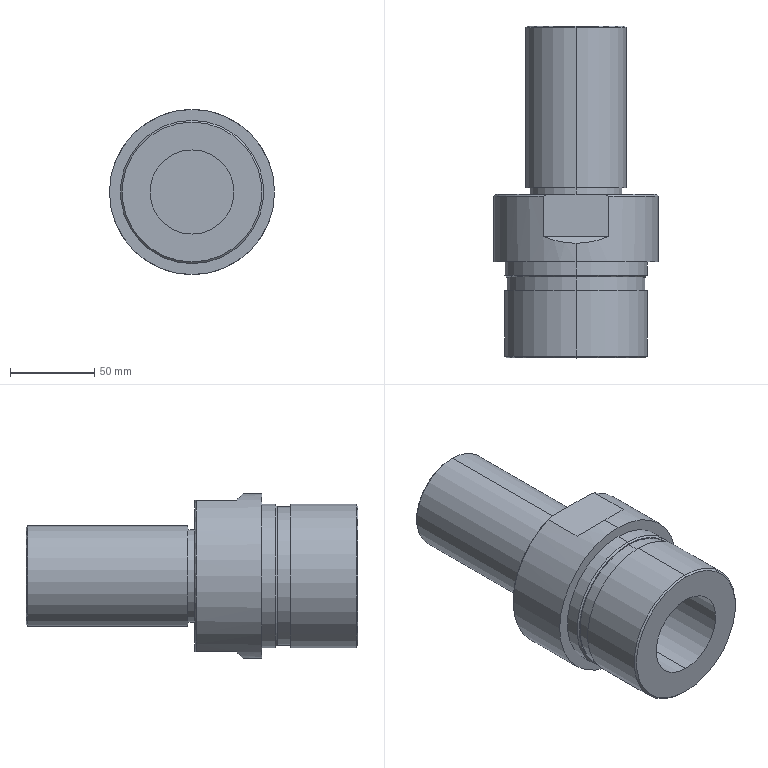Part | SolidWorks | features ICE 11, Chamfer 1, Extrusion 1 | 1 solid | 34 faces | box 98 x 197 x 98 mm | volume 798757 mm3 | cylinder 14 | plane 12 | cone 8 | commonest cylinder face diameters 85 x4 50 x2 55 x2 60 x2 82 x2 98 x2
STEP:
#1=CARTESIAN_POINT('',(0.,-7.,25.));
#2=VERTEX_POINT('',#1);
#3=CARTESIAN_POINT('',(0.,-7.,-25.));
#4=VERTEX_POINT('',#3);
#5=CARTESIAN_POINT('',(0.,-7.,0.));
#6=DIRECTION('',(0.,-1.,0.));
#7=DIRECTION('',(0.,0.,-1.));
#8=AXIS2_PLACEMENT_3D('',#5,#6,#7);
#9=CIRCLE('',#8,25.);
#10=EDGE_CURVE('',#2,#4,#9,.T.);
#11=ORIENTED_EDGE('',*,*,#10,.F.);
#12=CARTESIAN_POINT('',(0.,-57.,25.));
#13=VERTEX_POINT('',#12);
#14=CARTESIAN_POINT('',(0.,-7.,25.));
#15=DIRECTION('',(0.,-1.,0.));
#16=VECTOR('',#15,1000.);
#17=LINE('',#14,#16);
#18=EDGE_CURVE('',#2,#13,#17,.T.);
#19=ORIENTED_EDGE('',*,*,#18,.T.);
#20=CARTESIAN_POINT('',(0.,-57.,-25.));
#21=VERTEX_POINT('',#20);
#22=CARTESIAN_POINT('',(0.,-57.,0.));
#23=DIRECTION('',(0.,-1.,0.));
#24=DIRECTION('',(0.,0.,-1.));
#25=AXIS2_PLACEMENT_3D('',#22,#23,#24);
#26=CIRCLE('',#25,25.);
#27=EDGE_CURVE('',#13,#21,#26,.T.);
#28=ORIENTED_EDGE('',*,*,#27,.T.);
#29=CARTESIAN_POINT('',(0.,-7.,-25.));
#30=DIRECTION('',(0.,-1.,0.));
#31=VECTOR('',#30,1000.);
#32=LINE('',#29,#31);
#33=EDGE_CURVE('',#4,#21,#32,.T.);
#34=ORIENTED_EDGE('',*,*,#33,.F.);
#35=EDGE_LOOP('',(#11,#19,#28,#34));
#36=FACE_OUTER_BOUND('',#35,.T.);
#37=CARTESIAN_POINT('',(0.,-7.,0.));
#38=DIRECTION('',(0.,-1.,0.));
#39=DIRECTION('',(0.,0.,-1.));
#40=AXIS2_PLACEMENT_3D('',#37,#38,#39);
#41=CYLINDRICAL_SURFACE('',#40,25.);
#42=ADVANCED_FACE('',(#36),#41,.F.);
#43=CARTESIAN_POINT('',(0.,139.,-30.));
#44=VERTEX_POINT('',#43);
#45=CARTESIAN_POINT('',(0.,139.,30.));
#46=VERTEX_POINT('',#45);
#47=CARTESIAN_POINT('',(0.,139.,0.));
#48=DIRECTION('',(0.,-1.,0.));
#49=DIRECTION('',(0.,0.,1.));
#50=AXIS2_PLACEMENT_3D('',#47,#48,#49);
#51=CIRCLE('',#50,30.);
#52=EDGE_CURVE('',#44,#46,#51,.T.);
#53=ORIENTED_EDGE('',*,*,#52,.T.);
#54=CARTESIAN_POINT('',(0.,44.,30.));
#55=VERTEX_POINT('',#54);
#56=CARTESIAN_POINT('',(0.,140.,30.));
#57=DIRECTION('',(0.,-1.,0.));
#58=VECTOR('',#57,1000.);
#59=LINE('',#56,#58);
#60=EDGE_CURVE('',#46,#55,#59,.T.);
#61=ORIENTED_EDGE('',*,*,#60,.T.);
#62=CARTESIAN_POINT('',(0.,44.,-30.));
#63=VERTEX_POINT('',#62);
#64=CARTESIAN_POINT('',(0.,44.,0.));
#65=DIRECTION('',(0.,1.,0.));
#66=DIRECTION('',(0.,0.,1.));
#67=AXIS2_PLACEMENT_3D('',#64,#65,#66);
#68=CIRCLE('',#67,30.);
#69=EDGE_CURVE('',#55,#63,#68,.T.);
#70=ORIENTED_EDGE('',*,*,#69,.T.);
#71=CARTESIAN_POINT('',(0.,140.,-30.));
#72=DIRECTION('',(0.,-1.,0.));
#73=VECTOR('',#72,1000.);
#74=LINE('',#71,#73);
#75=EDGE_CURVE('',#44,#63,#74,.T.);
#76=ORIENTED_EDGE('',*,*,#75,.F.);
#77=EDGE_LOOP('',(#53,#61,#70,#76));
#78=FACE_OUTER_BOUND('',#77,.T.);
#79=CARTESIAN_POINT('',(0.,140.,0.));
#80=DIRECTION('',(0.,-1.,0.));
#81=DIRECTION('',(0.,0.,-1.));
#82=AXIS2_PLACEMENT_3D('',#79,#80,#81);
#83=CYLINDRICAL_SURFACE('',#82,30.);
#84=ADVANCED_FACE('',(#78),#83,.T.);
#85=CARTESIAN_POINT('',(0.,140.,29.));
#86=VERTEX_POINT('',#85);
#87=CARTESIAN_POINT('',(0.,140.,-29.));
#88=VERTEX_POINT('',#87);
#89=CARTESIAN_POINT('',(0.,140.,0.));
#90=DIRECTION('',(0.,1.,0.));
#91=DIRECTION('',(0.,0.,1.));
#92=AXIS2_PLACEMENT_3D('',#89,#90,#91);
#93=CIRCLE('',#92,29.);
#94=EDGE_CURVE('',#86,#88,#93,.T.);
#95=ORIENTED_EDGE('',*,*,#94,.F.);
#96=CARTESIAN_POINT('',(0.,140.,29.));
#97=DIRECTION('',(0.,-0.7071,0.7071));
#98=VECTOR('',#97,1000.);
#99=LINE('',#96,#98);
#100=EDGE_CURVE('',#86,#46,#99,.T.);
#101=ORIENTED_EDGE('',*,*,#100,.T.);
#102=ORIENTED_EDGE('',*,*,#52,.F.);
#103=CARTESIAN_POINT('',(0.,140.,-29.));
#104=DIRECTION('',(0.,-0.7071,-0.7071));
#105=VECTOR('',#104,1000.);
#106=LINE('',#103,#105);
#107=EDGE_CURVE('',#88,#44,#106,.T.);
#108=ORIENTED_EDGE('',*,*,#107,.F.);
#109=EDGE_LOOP('',(#95,#101,#102,#108));
#110=FACE_OUTER_BOUND('',#109,.T.);
#111=CARTESIAN_POINT('',(0.,140.,0.));
#112=DIRECTION('',(0.,-1.,0.));
#113=DIRECTION('',(0.,0.,-1.));
#114=AXIS2_PLACEMENT_3D('',#111,#112,#113);
#115=CONICAL_SURFACE('',#114,29.,0.7854);
#116=ADVANCED_FACE('',(#110),#115,.T.);
#117=CARTESIAN_POINT('',(0.,44.,27.5));
#118=VERTEX_POINT('',#117);
#119=CARTESIAN_POINT('',(0.,44.,-27.5));
#120=VERTEX_POINT('',#119);
#121=CARTESIAN_POINT('',(0.,44.,0.));
#122=DIRECTION('',(0.,1.,0.));
#123=DIRECTION('',(0.,0.,1.));
#124=AXIS2_PLACEMENT_3D('',#121,#122,#123);
#125=CIRCLE('',#124,27.5);
#126=EDGE_CURVE('',#118,#120,#125,.T.);
#127=ORIENTED_EDGE('',*,*,#126,.F.);
#128=CARTESIAN_POINT('',(0.,40.,27.5));
#129=VERTEX_POINT('',#128);
#130=CARTESIAN_POINT('',(0.,44.,27.5));
#131=DIRECTION('',(0.,-1.,0.));
#132=VECTOR('',#131,1000.);
#133=LINE('',#130,#132);
#134=EDGE_CURVE('',#118,#129,#133,.T.);
#135=ORIENTED_EDGE('',*,*,#134,.T.);
#136=CARTESIAN_POINT('',(0.,40.,-27.5));
#137=VERTEX_POINT('',#136);
#138=CARTESIAN_POINT('',(0.,40.,0.));
#139=DIRECTION('',(0.,1.,0.));
#140=DIRECTION('',(0.,0.,1.));
#141=AXIS2_PLACEMENT_3D('',#138,#139,#140);
#142=CIRCLE('',#141,27.5);
#143=EDGE_CURVE('',#129,#137,#142,.T.);
#144=ORIENTED_EDGE('',*,*,#143,.T.);
#145=CARTESIAN_POINT('',(0.,44.,-27.5));
#146=DIRECTION('',(0.,-1.,0.));
#147=VECTOR('',#146,1000.);
#148=LINE('',#145,#147);
#149=EDGE_CURVE('',#120,#137,#148,.T.);
#150=ORIENTED_EDGE('',*,*,#149,.F.);
#151=EDGE_LOOP('',(#127,#135,#144,#150));
#152=FACE_OUTER_BOUND('',#151,.T.);
#153=CARTESIAN_POINT('',(0.,44.,0.));
#154=DIRECTION('',(0.,-1.,0.));
#155=DIRECTION('',(0.,0.,-1.));
#156=AXIS2_PLACEMENT_3D('',#153,#154,#155);
#157=CYLINDRICAL_SURFACE('',#156,27.5);
#158=ADVANCED_FACE('',(#152),#157,.T.);
#159=CARTESIAN_POINT('',(0.,-9.,-41.5));
#160=VERTEX_POINT('',#159);
#161=CARTESIAN_POINT('',(0.,-9.,41.5));
#162=VERTEX_POINT('',#161);
#163=CARTESIAN_POINT('',(0.,-9.,0.));
#164=DIRECTION('',(0.,-1.,0.));
#165=DIRECTION('',(0.,0.,-1.));
#166=AXIS2_PLACEMENT_3D('',#163,#164,#165);
#167=CIRCLE('',#166,41.5);
#168=EDGE_CURVE('',#160,#162,#167,.T.);
#169=ORIENTED_EDGE('',*,*,#168,.F.);
#170=CARTESIAN_POINT('',(0.,-8.,-42.5));
#171=VERTEX_POINT('',#170);
#172=CARTESIAN_POINT('',(0.,-9.,-41.5));
#173=DIRECTION('',(0.,0.7071,-0.7071));
#174=VECTOR('',#173,1000.);
#175=LINE('',#172,#174);
#176=EDGE_CURVE('',#160,#171,#175,.T.);
#177=ORIENTED_EDGE('',*,*,#176,.T.);
#178=CARTESIAN_POINT('',(0.,-8.,42.5));
#179=VERTEX_POINT('',#178);
#180=CARTESIAN_POINT('',(0.,-8.,0.));
#181=DIRECTION('',(0.,1.,0.));
#182=DIRECTION('',(0.,0.,-1.));
#183=AXIS2_PLACEMENT_3D('',#180,#181,#182);
#184=CIRCLE('',#183,42.5);
#185=EDGE_CURVE('',#179,#171,#184,.T.);
#186=ORIENTED_EDGE('',*,*,#185,.F.);
#187=CARTESIAN_POINT('',(0.,-9.,41.5));
#188=DIRECTION('',(0.,0.7071,0.7071));
#189=VECTOR('',#188,1000.);
#190=LINE('',#187,#189);
#191=EDGE_CURVE('',#162,#179,#190,.T.);
#192=ORIENTED_EDGE('',*,*,#191,.F.);
#193=EDGE_LOOP('',(#169,#177,#186,#192));
#194=FACE_OUTER_BOUND('',#193,.T.);
#195=CARTESIAN_POINT('',(0.,-9.,0.));
#196=DIRECTION('',(0.,1.,0.));
#197=DIRECTION('',(0.,0.,1.));
#198=AXIS2_PLACEMENT_3D('',#195,#196,#197);
#199=CONICAL_SURFACE('',#198,41.5,0.7854);
#200=ADVANCED_FACE('',(#194),#199,.T.);
#201=CARTESIAN_POINT('',(0.,-57.,-41.5));
#202=VERTEX_POINT('',#201);
#203=CARTESIAN_POINT('',(0.,-57.,41.5));
#204=VERTEX_POINT('',#203);
#205=CARTESIAN_POINT('',(0.,-57.,0.));
#206=DIRECTION('',(0.,-1.,0.));
#207=DIRECTION('',(0.,0.,-1.));
#208=AXIS2_PLACEMENT_3D('',#205,#206,#207);
#209=CIRCLE('',#208,41.5);
#210=EDGE_CURVE('',#202,#204,#209,.T.);
#211=ORIENTED_EDGE('',*,*,#210,.F.);
#212=CARTESIAN_POINT('',(0.,-56.,-42.5));
#213=VERTEX_POINT('',#212);
#214=CARTESIAN_POINT('',(0.,-57.,-41.5));
#215=DIRECTION('',(0.,0.7071,-0.7071));
#216=VECTOR('',#215,1000.);
#217=LINE('',#214,#216);
#218=EDGE_CURVE('',#202,#213,#217,.T.);
#219=ORIENTED_EDGE('',*,*,#218,.T.);
#220=CARTESIAN_POINT('',(0.,-56.,42.5));
#221=VERTEX_POINT('',#220);
#222=CARTESIAN_POINT('',(0.,-56.,0.));
#223=DIRECTION('',(0.,1.,0.));
#224=DIRECTION('',(0.,0.,-1.));
#225=AXIS2_PLACEMENT_3D('',#222,#223,#224);
#226=CIRCLE('',#225,42.5);
#227=EDGE_CURVE('',#221,#213,#226,.T.);
#228=ORIENTED_EDGE('',*,*,#227,.F.);
#229=CARTESIAN_POINT('',(0.,-57.,41.5));
#230=DIRECTION('',(0.,0.7071,0.7071));
#231=VECTOR('',#230,1000.);
#232=LINE('',#229,#231);
#233=EDGE_CURVE('',#204,#221,#232,.T.);
#234=ORIENTED_EDGE('',*,*,#233,.F.);
#235=EDGE_LOOP('',(#211,#219,#228,#234));
#236=FACE_OUTER_BOUND('',#235,.T.);
#237=CARTESIAN_POINT('',(0.,-57.,0.));
#238=DIRECTION('',(0.,1.,0.));
#239=DIRECTION('',(0.,0.,1.));
#240=AXIS2_PLACEMENT_3D('',#237,#238,#239);
#241=CONICAL_SURFACE('',#240,41.5,0.7854);
#242=ADVANCED_FACE('',(#236),#241,.T.);
#243=ORIENTED_EDGE('',*,*,#227,.T.);
#244=CARTESIAN_POINT('',(0.,-17.,-42.5));
#245=VERTEX_POINT('',#244);
#246=CARTESIAN_POINT('',(0.,-57.,-42.5));
#247=DIRECTION('',(0.,1.,0.));
#248=VECTOR('',#247,1000.);
#249=LINE('',#246,#248);
#250=EDGE_CURVE('',#213,#245,#249,.T.);
#251=ORIENTED_EDGE('',*,*,#250,.T.);
#252=CARTESIAN_POINT('',(0.,-17.,42.5));
#253=VERTEX_POINT('',#252);
#254=CARTESIAN_POINT('',(0.,-17.,0.));
#255=DIRECTION('',(0.,-1.,0.));
#256=DIRECTION('',(0.,0.,-1.));
#257=AXIS2_PLACEMENT_3D('',#254,#255,#256);
#258=CIRCLE('',#257,42.5);
#259=EDGE_CURVE('',#245,#253,#258,.T.);
#260=ORIENTED_EDGE('',*,*,#259,.T.);
#261=CARTESIAN_POINT('',(0.,-57.,42.5));
#262=DIRECTION('',(0.,1.,0.));
#263=VECTOR('',#262,1000.);
#264=LINE('',#261,#263);
#265=EDGE_CURVE('',#221,#253,#264,.T.);
#266=ORIENTED_EDGE('',*,*,#265,.F.);
#267=EDGE_LOOP('',(#243,#251,#260,#266));
#268=FACE_OUTER_BOUND('',#267,.T.);
#269=CARTESIAN_POINT('',(0.,-57.,0.));
#270=DIRECTION('',(0.,1.,0.));
#271=DIRECTION('',(0.,0.,1.));
#272=AXIS2_PLACEMENT_3D('',#269,#270,#271);
#273=CYLINDRICAL_SURFACE('',#272,42.5);
#274=ADVANCED_FACE('',(#268),#273,.T.);
#275=CARTESIAN_POINT('',(0.,-17.,-41.));
#276=VERTEX_POINT('',#275);
#277=CARTESIAN_POINT('',(0.,-17.,41.));
#278=VERTEX_POINT('',#277);
#279=CARTESIAN_POINT('',(0.,-17.,0.));
#280=DIRECTION('',(0.,-1.,0.));
#281=DIRECTION('',(0.,0.,-1.));
#282=AXIS2_PLACEMENT_3D('',#279,#280,#281);
#283=CIRCLE('',#282,41.);
#284=EDGE_CURVE('',#276,#278,#283,.T.);
#285=ORIENTED_EDGE('',*,*,#284,.F.);
#286=CARTESIAN_POINT('',(0.,-9.,-41.));
#287=VERTEX_POINT('',#286);
#288=CARTESIAN_POINT('',(0.,-17.,-41.));
#289=DIRECTION('',(0.,1.,0.));
#290=VECTOR('',#289,1000.);
#291=LINE('',#288,#290);
#292=EDGE_CURVE('',#276,#287,#291,.T.);
#293=ORIENTED_EDGE('',*,*,#292,.T.);
#294=CARTESIAN_POINT('',(0.,-9.,41.));
#295=VERTEX_POINT('',#294);
#296=CARTESIAN_POINT('',(0.,-9.,0.));
#297=DIRECTION('',(0.,-1.,0.));
#298=DIRECTION('',(0.,0.,-1.));
#299=AXIS2_PLACEMENT_3D('',#296,#297,#298);
#300=CIRCLE('',#299,41.);
#301=EDGE_CURVE('',#287,#295,#300,.T.);
#302=ORIENTED_EDGE('',*,*,#301,.T.);
#303=CARTESIAN_POINT('',(0.,-17.,41.));
#304=DIRECTION('',(0.,1.,0.));
#305=VECTOR('',#304,1000.);
#306=LINE('',#303,#305);
#307=EDGE_CURVE('',#278,#295,#306,.T.);
#308=ORIENTED_EDGE('',*,*,#307,.F.);
#309=EDGE_LOOP('',(#285,#293,#302,#308));
#310=FACE_OUTER_BOUND('',#309,.T.);
#311=CARTESIAN_POINT('',(0.,-17.,0.));
#312=DIRECTION('',(0.,1.,0.));
#313=DIRECTION('',(0.,0.,1.));
#314=AXIS2_PLACEMENT_3D('',#311,#312,#313);
#315=CYLINDRICAL_SURFACE('',#314,41.);
#316=ADVANCED_FACE('',(#310),#315,.T.);
#317=ORIENTED_EDGE('',*,*,#185,.T.);
#318=CARTESIAN_POINT('',(0.,0.,-42.5));
#319=VERTEX_POINT('',#318);
#320=CARTESIAN_POINT('',(0.,-9.,-42.5));
#321=DIRECTION('',(0.,1.,0.));
#322=VECTOR('',#321,1000.);
#323=LINE('',#320,#322);
#324=EDGE_CURVE('',#171,#319,#323,.T.);
#325=ORIENTED_EDGE('',*,*,#324,.T.);
#326=CARTESIAN_POINT('',(0.,0.,42.5));
#327=VERTEX_POINT('',#326);
#328=CARTESIAN_POINT('',(0.,0.,0.));
#329=DIRECTION('',(0.,-1.,0.));
#330=DIRECTION('',(0.,0.,1.));
#331=AXIS2_PLACEMENT_3D('',#328,#329,#330);
#332=CIRCLE('',#331,42.5);
#333=EDGE_CURVE('',#319,#327,#332,.T.);
#334=ORIENTED_EDGE('',*,*,#333,.T.);
#335=CARTESIAN_POINT('',(0.,-9.,42.5));
#336=DIRECTION('',(0.,1.,0.));
#337=VECTOR('',#336,1000.);
#338=LINE('',#335,#337);
#339=EDGE_CURVE('',#179,#327,#338,.T.);
#340=ORIENTED_EDGE('',*,*,#339,.F.);
#341=EDGE_LOOP('',(#317,#325,#334,#340));
#342=FACE_OUTER_BOUND('',#341,.T.);
#343=CARTESIAN_POINT('',(0.,-9.,0.));
#344=DIRECTION('',(0.,1.,0.));
#345=DIRECTION('',(0.,0.,1.));
#346=AXIS2_PLACEMENT_3D('',#343,#344,#345);
#347=CYLINDRICAL_SURFACE('',#346,42.5);
#348=ADVANCED_FACE('',(#342),#347,.T.);
#349=CARTESIAN_POINT('',(19.391,15.,45.));
#350=VERTEX_POINT('',#349);
#351=CARTESIAN_POINT('',(0.,11.,49.));
#352=VERTEX_POINT('',#351);
#353=CARTESIAN_POINT('',(19.391,15.,45.));
#354=CARTESIAN_POINT('',(13.245,12.352,47.648));
#355=CARTESIAN_POINT('',(6.692,11.,49.));
#356=CARTESIAN_POINT('',(0.,11.,49.));
#357=(BOUNDED_CURVE()B_SPLINE_CURVE(3,(#353,#354,#355,#356),.UNSPECIFIED.,.F.,.F.)B_SPLINE_CURVE_WITH_KNOTS((4,4),(5.876,6.283),.UNSPECIFIED.)CURVE()GEOMETRIC_REPRESENTATION_ITEM()RATIONAL_B_SPLINE_CURVE((1.,0.9863,0.9863,1.))REPRESENTATION_ITEM(''));
#358=EDGE_CURVE('',#350,#352,#357,.T.);
#359=ORIENTED_EDGE('',*,*,#358,.T.);
#360=CARTESIAN_POINT('',(0.,0.,49.));
#361=VERTEX_POINT('',#360);
#362=CARTESIAN_POINT('',(0.,40.,49.));
#363=DIRECTION('',(0.,-1.,0.));
#364=VECTOR('',#363,1000.);
#365=LINE('',#362,#364);
#366=EDGE_CURVE('',#352,#361,#365,.T.);
#367=ORIENTED_EDGE('',*,*,#366,.T.);
#368=CARTESIAN_POINT('',(0.,0.,-49.));
#369=VERTEX_POINT('',#368);
#370=CARTESIAN_POINT('',(0.,0.,0.));
#371=DIRECTION('',(0.,1.,0.));
#372=DIRECTION('',(0.,0.,1.));
#373=AXIS2_PLACEMENT_3D('',#370,#371,#372);
#374=CIRCLE('',#373,49.);
#375=EDGE_CURVE('',#361,#369,#374,.T.);
#376=ORIENTED_EDGE('',*,*,#375,.T.);
#377=CARTESIAN_POINT('',(0.,11.,-49.));
#378=VERTEX_POINT('',#377);
#379=CARTESIAN_POINT('',(0.,40.,-49.));
#380=DIRECTION('',(0.,-1.,0.));
#381=VECTOR('',#380,1000.);
#382=LINE('',#379,#381);
#383=EDGE_CURVE('',#378,#369,#382,.T.);
#384=ORIENTED_EDGE('',*,*,#383,.F.);
#385=CARTESIAN_POINT('',(19.391,15.,-45.));
#386=VERTEX_POINT('',#385);
#387=CARTESIAN_POINT('',(0.,11.,-49.));
#388=CARTESIAN_POINT('',(6.692,11.,-49.));
#389=CARTESIAN_POINT('',(13.245,12.352,-47.648));
#390=CARTESIAN_POINT('',(19.391,15.,-45.));
#391=(BOUNDED_CURVE()B_SPLINE_CURVE(3,(#387,#388,#389,#390),.UNSPECIFIED.,.F.,.F.)B_SPLINE_CURVE_WITH_KNOTS((4,4),(0.,0.4069),.UNSPECIFIED.)CURVE()GEOMETRIC_REPRESENTATION_ITEM()RATIONAL_B_SPLINE_CURVE((1.,0.9863,0.9863,1.))REPRESENTATION_ITEM(''));
#392=EDGE_CURVE('',#378,#386,#391,.T.);
#393=ORIENTED_EDGE('',*,*,#392,.T.);
#394=CARTESIAN_POINT('',(19.391,39.,-45.));
#395=VERTEX_POINT('',#394);
#396=CARTESIAN_POINT('',(19.391,40.,-45.));
#397=DIRECTION('',(0.,1.,0.));
#398=VECTOR('',#397,1000.);
#399=LINE('',#396,#398);
#400=EDGE_CURVE('',#386,#395,#399,.T.);
#401=ORIENTED_EDGE('',*,*,#400,.T.);
#402=CARTESIAN_POINT('',(19.391,39.,45.));
#403=VERTEX_POINT('',#402);
#404=CARTESIAN_POINT('',(0.,39.,0.));
#405=DIRECTION('',(0.,-1.,0.));
#406=DIRECTION('',(0.,0.,1.));
#407=AXIS2_PLACEMENT_3D('',#404,#405,#406);
#408=CIRCLE('',#407,49.);
#409=EDGE_CURVE('',#395,#403,#408,.T.);
#410=ORIENTED_EDGE('',*,*,#409,.T.);
#411=CARTESIAN_POINT('',(19.391,40.,45.));
#412=DIRECTION('',(0.,-1.,0.));
#413=VECTOR('',#412,1000.);
#414=LINE('',#411,#413);
#415=EDGE_CURVE('',#403,#350,#414,.T.);
#416=ORIENTED_EDGE('',*,*,#415,.T.);
#417=EDGE_LOOP('',(#359,#367,#376,#384,#393,#401,#410,#416));
#418=FACE_OUTER_BOUND('',#417,.T.);
#419=CARTESIAN_POINT('',(0.,40.,0.));
#420=DIRECTION('',(0.,-1.,0.));
#421=DIRECTION('',(0.,0.,-1.));
#422=AXIS2_PLACEMENT_3D('',#419,#420,#421);
#423=CYLINDRICAL_SURFACE('',#422,49.);
#424=ADVANCED_FACE('',(#418),#423,.T.);
#425=ORIENTED_EDGE('',*,*,#366,.F.);
#426=CARTESIAN_POINT('',(-19.391,15.,45.));
#427=VERTEX_POINT('',#426);
#428=CARTESIAN_POINT('',(0.,11.,49.));
#429=CARTESIAN_POINT('',(-6.692,11.,49.));
#430=CARTESIAN_POINT('',(-13.245,12.352,47.648));
#431=CARTESIAN_POINT('',(-19.391,15.,45.));
#432=(BOUNDED_CURVE()B_SPLINE_CURVE(3,(#428,#429,#430,#431),.UNSPECIFIED.,.F.,.F.)B_SPLINE_CURVE_WITH_KNOTS((4,4),(0.,0.4069),.UNSPECIFIED.)CURVE()GEOMETRIC_REPRESENTATION_ITEM()RATIONAL_B_SPLINE_CURVE((1.,0.9863,0.9863,1.))REPRESENTATION_ITEM(''));
#433=EDGE_CURVE('',#352,#427,#432,.T.);
#434=ORIENTED_EDGE('',*,*,#433,.T.);
#435=CARTESIAN_POINT('',(-19.391,39.,45.));
#436=VERTEX_POINT('',#435);
#437=CARTESIAN_POINT('',(-19.391,40.,45.));
#438=DIRECTION('',(0.,1.,0.));
#439=VECTOR('',#438,1000.);
#440=LINE('',#437,#439);
#441=EDGE_CURVE('',#427,#436,#440,.T.);
#442=ORIENTED_EDGE('',*,*,#441,.T.);
#443=CARTESIAN_POINT('',(-19.391,39.,-45.));
#444=VERTEX_POINT('',#443);
#445=CARTESIAN_POINT('',(0.,39.,0.));
#446=DIRECTION('',(0.,-1.,0.));
#447=DIRECTION('',(0.,0.,1.));
#448=AXIS2_PLACEMENT_3D('',#445,#446,#447);
#449=CIRCLE('',#448,49.);
#450=EDGE_CURVE('',#436,#444,#449,.T.);
#451=ORIENTED_EDGE('',*,*,#450,.T.);
#452=CARTESIAN_POINT('',(-19.391,15.,-45.));
#453=VERTEX_POINT('',#452);
#454=CARTESIAN_POINT('',(-19.391,40.,-45.));
#455=DIRECTION('',(0.,-1.,0.));
#456=VECTOR('',#455,1000.);
#457=LINE('',#454,#456);
#458=EDGE_CURVE('',#444,#453,#457,.T.);
#459=ORIENTED_EDGE('',*,*,#458,.T.);
#460=CARTESIAN_POINT('',(-19.391,15.,-45.));
#461=CARTESIAN_POINT('',(-13.245,12.352,-47.648));
#462=CARTESIAN_POINT('',(-6.692,11.,-49.));
#463=CARTESIAN_POINT('',(0.,11.,-49.));
#464=(BOUNDED_CURVE()B_SPLINE_CURVE(3,(#460,#461,#462,#463),.UNSPECIFIED.,.F.,.F.)B_SPLINE_CURVE_WITH_KNOTS((4,4),(5.876,6.283),.UNSPECIFIED.)CURVE()GEOMETRIC_REPRESENTATION_ITEM()RATIONAL_B_SPLINE_CURVE((1.,0.9863,0.9863,1.))REPRESENTATION_ITEM(''));
#465=EDGE_CURVE('',#453,#378,#464,.T.);
#466=ORIENTED_EDGE('',*,*,#465,.T.);
#467=ORIENTED_EDGE('',*,*,#383,.T.);
#468=CARTESIAN_POINT('',(0.,0.,0.));
#469=DIRECTION('',(0.,1.,0.));
#470=DIRECTION('',(0.,0.,1.));
#471=AXIS2_PLACEMENT_3D('',#468,#469,#470);
#472=CIRCLE('',#471,49.);
#473=EDGE_CURVE('',#369,#361,#472,.T.);
#474=ORIENTED_EDGE('',*,*,#473,.T.);
#475=EDGE_LOOP('',(#425,#434,#442,#451,#459,#466,#467,#474));
#476=FACE_OUTER_BOUND('',#475,.T.);
#477=CARTESIAN_POINT('',(0.,40.,0.));
#478=DIRECTION('',(0.,-1.,0.));
#479=DIRECTION('',(0.,0.,-1.));
#480=AXIS2_PLACEMENT_3D('',#477,#478,#479);
#481=CYLINDRICAL_SURFACE('',#480,49.);
#482=ADVANCED_FACE('',(#476),#481,.T.);
#483=CARTESIAN_POINT('',(16.703,40.,45.));
#484=VERTEX_POINT('',#483);
#485=CARTESIAN_POINT('',(19.391,39.,45.));
#486=CARTESIAN_POINT('',(18.502,39.352,45.));
#487=CARTESIAN_POINT('',(17.607,39.686,45.));
#488=CARTESIAN_POINT('',(16.703,40.,45.));
#489=B_SPLINE_CURVE_WITH_KNOTS('',3,(#485,#486,#487,#488),.UNSPECIFIED.,.F.,.F.,(4,4),(0.09858,0.1015),.UNSPECIFIED.);
#490=EDGE_CURVE('',#403,#484,#489,.T.);
#491=ORIENTED_EDGE('',*,*,#490,.F.);
#492=ORIENTED_EDGE('',*,*,#409,.F.);
#493=CARTESIAN_POINT('',(16.703,40.,-45.));
#494=VERTEX_POINT('',#493);
#495=CARTESIAN_POINT('',(16.703,40.,-45.));
#496=CARTESIAN_POINT('',(17.604,39.687,-45.));
#497=CARTESIAN_POINT('',(18.5,39.353,-45.));
#498=CARTESIAN_POINT('',(19.391,39.,-45.));
#499=B_SPLINE_CURVE_WITH_KNOTS('',3,(#495,#496,#497,#498),.UNSPECIFIED.,.F.,.F.,(4,4),(0.1355,0.1384),.UNSPECIFIED.);
#500=EDGE_CURVE('',#494,#395,#499,.T.);
#501=ORIENTED_EDGE('',*,*,#500,.F.);
#502=CARTESIAN_POINT('',(0.,40.,0.));
#503=DIRECTION('',(0.,1.,0.));
#504=DIRECTION('',(0.,0.,1.));
#505=AXIS2_PLACEMENT_3D('',#502,#503,#504);
#506=CIRCLE('',#505,48.);
#507=EDGE_CURVE('',#484,#494,#506,.T.);
#508=ORIENTED_EDGE('',*,*,#507,.F.);
#509=EDGE_LOOP('',(#491,#492,#501,#508));
#510=FACE_OUTER_BOUND('',#509,.T.);
#511=CARTESIAN_POINT('',(0.,40.,0.));
#512=DIRECTION('',(0.,-1.,0.));
#513=DIRECTION('',(0.,0.,-1.));
#514=AXIS2_PLACEMENT_3D('',#511,#512,#513);
#515=CONICAL_SURFACE('',#514,48.,0.7854);
#516=ADVANCED_FACE('',(#510),#515,.T.);
#517=CARTESIAN_POINT('',(0.,-9.,0.));
#518=DIRECTION('',(0.,-1.,0.));
#519=DIRECTION('',(0.,0.,-1.));
#520=AXIS2_PLACEMENT_3D('',#517,#518,#519);
#521=CIRCLE('',#520,41.5);
#522=EDGE_CURVE('',#162,#160,#521,.T.);
#523=ORIENTED_EDGE('',*,*,#522,.T.);
#524=ORIENTED_EDGE('',*,*,#168,.T.);
#525=EDGE_LOOP('',(#523,#524));
#526=FACE_OUTER_BOUND('',#525,.T.);
#527=CARTESIAN_POINT('',(0.,-9.,0.));
#528=DIRECTION('',(0.,-1.,0.));
#529=DIRECTION('',(0.,0.,-1.));
#530=AXIS2_PLACEMENT_3D('',#527,#528,#529);
#531=CIRCLE('',#530,41.);
#532=EDGE_CURVE('',#295,#287,#531,.T.);
#533=ORIENTED_EDGE('',*,*,#532,.F.);
#534=ORIENTED_EDGE('',*,*,#301,.F.);
#535=EDGE_LOOP('',(#533,#534));
#536=FACE_BOUND('',#535,.T.);
#537=CARTESIAN_POINT('',(0.,-9.,0.));
#538=DIRECTION('',(0.,-1.,0.));
#539=DIRECTION('',(0.,0.,-1.));
#540=AXIS2_PLACEMENT_3D('',#537,#538,#539);
#541=PLANE('',#540);
#542=ADVANCED_FACE('',(#526,#536),#541,.T.);
#543=ORIENTED_EDGE('',*,*,#473,.F.);
#544=ORIENTED_EDGE('',*,*,#375,.F.);
#545=EDGE_LOOP('',(#543,#544));
#546=FACE_OUTER_BOUND('',#545,.T.);
#547=CARTESIAN_POINT('',(0.,0.,0.));
#548=DIRECTION('',(0.,-1.,0.));
#549=DIRECTION('',(0.,0.,1.));
#550=AXIS2_PLACEMENT_3D('',#547,#548,#549);
#551=CIRCLE('',#550,42.5);
#552=EDGE_CURVE('',#327,#319,#551,.T.);
#553=ORIENTED_EDGE('',*,*,#552,.F.);
#554=ORIENTED_EDGE('',*,*,#333,.F.);
#555=EDGE_LOOP('',(#553,#554));
#556=FACE_BOUND('',#555,.T.);
#557=CARTESIAN_POINT('',(0.,0.,0.));
#558=DIRECTION('',(0.,1.,0.));
#559=DIRECTION('',(0.,0.,1.));
#560=AXIS2_PLACEMENT_3D('',#557,#558,#559);
#561=PLANE('',#560);
#562=ADVANCED_FACE('',(#546,#556),#561,.F.);
#563=CARTESIAN_POINT('',(-16.703,40.,45.));
#564=VERTEX_POINT('',#563);
#565=CARTESIAN_POINT('',(-77.,40.,45.));
#566=DIRECTION('',(-1.,0.,0.));
#567=VECTOR('',#566,1000.);
#568=LINE('',#565,#567);
#569=EDGE_CURVE('',#484,#564,#568,.T.);
#570=ORIENTED_EDGE('',*,*,#569,.F.);
#571=ORIENTED_EDGE('',*,*,#507,.T.);
#572=CARTESIAN_POINT('',(-16.703,40.,-45.));
#573=VERTEX_POINT('',#572);
#574=CARTESIAN_POINT('',(-77.,40.,-45.));
#575=DIRECTION('',(1.,0.,0.));
#576=VECTOR('',#575,1000.);
#577=LINE('',#574,#576);
#578=EDGE_CURVE('',#573,#494,#577,.T.);
#579=ORIENTED_EDGE('',*,*,#578,.F.);
#580=CARTESIAN_POINT('',(0.,40.,0.));
#581=DIRECTION('',(0.,1.,0.));
#582=DIRECTION('',(0.,0.,1.));
#583=AXIS2_PLACEMENT_3D('',#580,#581,#582);
#584=CIRCLE('',#583,48.);
#585=EDGE_CURVE('',#573,#564,#584,.T.);
#586=ORIENTED_EDGE('',*,*,#585,.T.);
#587=EDGE_LOOP('',(#570,#571,#579,#586));
#588=FACE_OUTER_BOUND('',#587,.T.);
#589=CARTESIAN_POINT('',(0.,40.,0.));
#590=DIRECTION('',(0.,1.,0.));
#591=DIRECTION('',(0.,0.,1.));
#592=AXIS2_PLACEMENT_3D('',#589,#590,#591);
#593=CIRCLE('',#592,27.5);
#594=EDGE_CURVE('',#137,#129,#593,.T.);
#595=ORIENTED_EDGE('',*,*,#594,.F.);
#596=ORIENTED_EDGE('',*,*,#143,.F.);
#597=EDGE_LOOP('',(#595,#596));
#598=FACE_BOUND('',#597,.T.);
#599=CARTESIAN_POINT('',(0.,40.,0.));
#600=DIRECTION('',(0.,1.,0.));
#601=DIRECTION('',(0.,0.,1.));
#602=AXIS2_PLACEMENT_3D('',#599,#600,#601);
#603=PLANE('',#602);
#604=ADVANCED_FACE('',(#588,#598),#603,.T.);
#605=ORIENTED_EDGE('',*,*,#324,.F.);
#606=CARTESIAN_POINT('',(0.,-8.,0.));
#607=DIRECTION('',(0.,1.,0.));
#608=DIRECTION('',(0.,0.,-1.));
#609=AXIS2_PLACEMENT_3D('',#606,#607,#608);
#610=CIRCLE('',#609,42.5);
#611=EDGE_CURVE('',#171,#179,#610,.T.);
#612=ORIENTED_EDGE('',*,*,#611,.T.);
#613=ORIENTED_EDGE('',*,*,#339,.T.);
#614=ORIENTED_EDGE('',*,*,#552,.T.);
#615=EDGE_LOOP('',(#605,#612,#613,#614));
#616=FACE_OUTER_BOUND('',#615,.T.);
#617=CARTESIAN_POINT('',(0.,-9.,0.));
#618=DIRECTION('',(0.,1.,0.));
#619=DIRECTION('',(0.,0.,1.));
#620=AXIS2_PLACEMENT_3D('',#617,#618,#619);
#621=CYLINDRICAL_SURFACE('',#620,42.5);
#622=ADVANCED_FACE('',(#616),#621,.T.);
#623=ORIENTED_EDGE('',*,*,#292,.F.);
#624=CARTESIAN_POINT('',(0.,-17.,0.));
#625=DIRECTION('',(0.,-1.,0.));
#626=DIRECTION('',(0.,0.,-1.));
#627=AXIS2_PLACEMENT_3D('',#624,#625,#626);
#628=CIRCLE('',#627,41.);
#629=EDGE_CURVE('',#278,#276,#628,.T.);
#630=ORIENTED_EDGE('',*,*,#629,.F.);
#631=ORIENTED_EDGE('',*,*,#307,.T.);
#632=ORIENTED_EDGE('',*,*,#532,.T.);
#633=EDGE_LOOP('',(#623,#630,#631,#632));
#634=FACE_OUTER_BOUND('',#633,.T.);
#635=CARTESIAN_POINT('',(0.,-17.,0.));
#636=DIRECTION('',(0.,1.,0.));
#637=DIRECTION('',(0.,0.,1.));
#638=AXIS2_PLACEMENT_3D('',#635,#636,#637);
#639=CYLINDRICAL_SURFACE('',#638,41.);
#640=ADVANCED_FACE('',(#634),#639,.T.);
#641=CARTESIAN_POINT('',(0.,-17.,0.));
#642=DIRECTION('',(0.,-1.,0.));
#643=DIRECTION('',(0.,0.,-1.));
#644=AXIS2_PLACEMENT_3D('',#641,#642,#643);
#645=CIRCLE('',#644,42.5);
#646=EDGE_CURVE('',#253,#245,#645,.T.);
#647=ORIENTED_EDGE('',*,*,#646,.F.);
#648=ORIENTED_EDGE('',*,*,#259,.F.);
#649=EDGE_LOOP('',(#647,#648));
#650=FACE_OUTER_BOUND('',#649,.T.);
#651=ORIENTED_EDGE('',*,*,#629,.T.);
#652=ORIENTED_EDGE('',*,*,#284,.T.);
#653=EDGE_LOOP('',(#651,#652));
#654=FACE_BOUND('',#653,.T.);
#655=CARTESIAN_POINT('',(0.,-17.,0.));
#656=DIRECTION('',(0.,-1.,0.));
#657=DIRECTION('',(0.,0.,-1.));
#658=AXIS2_PLACEMENT_3D('',#655,#656,#657);
#659=PLANE('',#658);
#660=ADVANCED_FACE('',(#650,#654),#659,.F.);
#661=ORIENTED_EDGE('',*,*,#250,.F.);
#662=CARTESIAN_POINT('',(0.,-56.,0.));
#663=DIRECTION('',(0.,1.,0.));
#664=DIRECTION('',(0.,0.,-1.));
#665=AXIS2_PLACEMENT_3D('',#662,#663,#664);
#666=CIRCLE('',#665,42.5);
#667=EDGE_CURVE('',#213,#221,#666,.T.);
#668=ORIENTED_EDGE('',*,*,#667,.T.);
#669=ORIENTED_EDGE('',*,*,#265,.T.);
#670=ORIENTED_EDGE('',*,*,#646,.T.);
#671=EDGE_LOOP('',(#661,#668,#669,#670));
#672=FACE_OUTER_BOUND('',#671,.T.);
#673=CARTESIAN_POINT('',(0.,-57.,0.));
#674=DIRECTION('',(0.,1.,0.));
#675=DIRECTION('',(0.,0.,1.));
#676=AXIS2_PLACEMENT_3D('',#673,#674,#675);
#677=CYLINDRICAL_SURFACE('',#676,42.5);
#678=ADVANCED_FACE('',(#672),#677,.T.);
#679=CARTESIAN_POINT('',(0.,-57.,0.));
#680=DIRECTION('',(0.,-1.,0.));
#681=DIRECTION('',(0.,0.,-1.));
#682=AXIS2_PLACEMENT_3D('',#679,#680,#681);
#683=CIRCLE('',#682,25.);
#684=EDGE_CURVE('',#21,#13,#683,.T.);
#685=ORIENTED_EDGE('',*,*,#684,.F.);
#686=ORIENTED_EDGE('',*,*,#27,.F.);
#687=EDGE_LOOP('',(#685,#686));
#688=FACE_BOUND('',#687,.T.);
#689=CARTESIAN_POINT('',(0.,-57.,0.));
#690=DIRECTION('',(0.,-1.,0.));
#691=DIRECTION('',(0.,0.,-1.));
#692=AXIS2_PLACEMENT_3D('',#689,#690,#691);
#693=CIRCLE('',#692,41.5);
#694=EDGE_CURVE('',#204,#202,#693,.T.);
#695=ORIENTED_EDGE('',*,*,#694,.T.);
#696=ORIENTED_EDGE('',*,*,#210,.T.);
#697=EDGE_LOOP('',(#695,#696));
#698=FACE_OUTER_BOUND('',#697,.T.);
#699=CARTESIAN_POINT('',(0.,-57.,0.));
#700=DIRECTION('',(0.,-1.,0.));
#701=DIRECTION('',(0.,0.,-1.));
#702=AXIS2_PLACEMENT_3D('',#699,#700,#701);
#703=PLANE('',#702);
#704=ADVANCED_FACE('',(#688,#698),#703,.T.);
#705=CARTESIAN_POINT('',(-16.703,40.,45.));
#706=CARTESIAN_POINT('',(-17.604,39.687,45.));
#707=CARTESIAN_POINT('',(-18.5,39.353,45.));
#708=CARTESIAN_POINT('',(-19.391,39.,45.));
#709=B_SPLINE_CURVE_WITH_KNOTS('',3,(#705,#706,#707,#708),.UNSPECIFIED.,.F.,.F.,(4,4),(0.1355,0.1384),.UNSPECIFIED.);
#710=EDGE_CURVE('',#564,#436,#709,.T.);
#711=ORIENTED_EDGE('',*,*,#710,.F.);
#712=ORIENTED_EDGE('',*,*,#585,.F.);
#713=CARTESIAN_POINT('',(-19.391,39.,-45.));
#714=CARTESIAN_POINT('',(-18.502,39.352,-45.));
#715=CARTESIAN_POINT('',(-17.607,39.686,-45.));
#716=CARTESIAN_POINT('',(-16.703,40.,-45.));
#717=B_SPLINE_CURVE_WITH_KNOTS('',3,(#713,#714,#715,#716),.UNSPECIFIED.,.F.,.F.,(4,4),(0.09858,0.1015),.UNSPECIFIED.);
#718=EDGE_CURVE('',#444,#573,#717,.T.);
#719=ORIENTED_EDGE('',*,*,#718,.F.);
#720=ORIENTED_EDGE('',*,*,#450,.F.);
#721=EDGE_LOOP('',(#711,#712,#719,#720));
#722=FACE_OUTER_BOUND('',#721,.T.);
#723=CARTESIAN_POINT('',(0.,40.,0.));
#724=DIRECTION('',(0.,-1.,0.));
#725=DIRECTION('',(0.,0.,-1.));
#726=AXIS2_PLACEMENT_3D('',#723,#724,#725);
#727=CONICAL_SURFACE('',#726,48.,0.7854);
#728=ADVANCED_FACE('',(#722),#727,.T.);
#729=ORIENTED_EDGE('',*,*,#218,.F.);
#730=ORIENTED_EDGE('',*,*,#694,.F.);
#731=ORIENTED_EDGE('',*,*,#233,.T.);
#732=ORIENTED_EDGE('',*,*,#667,.F.);
#733=EDGE_LOOP('',(#729,#730,#731,#732));
#734=FACE_OUTER_BOUND('',#733,.T.);
#735=CARTESIAN_POINT('',(0.,-57.,0.));
#736=DIRECTION('',(0.,1.,0.));
#737=DIRECTION('',(0.,0.,1.));
#738=AXIS2_PLACEMENT_3D('',#735,#736,#737);
#739=CONICAL_SURFACE('',#738,41.5,0.7854);
#740=ADVANCED_FACE('',(#734),#739,.T.);
#741=ORIENTED_EDGE('',*,*,#176,.F.);
#742=ORIENTED_EDGE('',*,*,#522,.F.);
#743=ORIENTED_EDGE('',*,*,#191,.T.);
#744=ORIENTED_EDGE('',*,*,#611,.F.);
#745=EDGE_LOOP('',(#741,#742,#743,#744));
#746=FACE_OUTER_BOUND('',#745,.T.);
#747=CARTESIAN_POINT('',(0.,-9.,0.));
#748=DIRECTION('',(0.,1.,0.));
#749=DIRECTION('',(0.,0.,1.));
#750=AXIS2_PLACEMENT_3D('',#747,#748,#749);
#751=CONICAL_SURFACE('',#750,41.5,0.7854);
#752=ADVANCED_FACE('',(#746),#751,.T.);
#753=ORIENTED_EDGE('',*,*,#718,.T.);
#754=ORIENTED_EDGE('',*,*,#578,.T.);
#755=ORIENTED_EDGE('',*,*,#500,.T.);
#756=ORIENTED_EDGE('',*,*,#400,.F.);
#757=CARTESIAN_POINT('',(-77.,15.,-45.));
#758=DIRECTION('',(1.,0.,0.));
#759=VECTOR('',#758,1000.);
#760=LINE('',#757,#759);
#761=EDGE_CURVE('',#453,#386,#760,.T.);
#762=ORIENTED_EDGE('',*,*,#761,.F.);
#763=ORIENTED_EDGE('',*,*,#458,.F.);
#764=EDGE_LOOP('',(#753,#754,#755,#756,#762,#763));
#765=FACE_OUTER_BOUND('',#764,.T.);
#766=CARTESIAN_POINT('',(-77.,15.,-45.));
#767=DIRECTION('',(0.,0.,1.));
#768=DIRECTION('',(1.,0.,0.));
#769=AXIS2_PLACEMENT_3D('',#766,#767,#768);
#770=PLANE('',#769);
#771=ADVANCED_FACE('',(#765),#770,.F.);
#772=ORIENTED_EDGE('',*,*,#490,.T.);
#773=ORIENTED_EDGE('',*,*,#569,.T.);
#774=ORIENTED_EDGE('',*,*,#710,.T.);
#775=ORIENTED_EDGE('',*,*,#441,.F.);
#776=CARTESIAN_POINT('',(-77.,15.,45.));
#777=DIRECTION('',(-1.,0.,0.));
#778=VECTOR('',#777,1000.);
#779=LINE('',#776,#778);
#780=EDGE_CURVE('',#350,#427,#779,.T.);
#781=ORIENTED_EDGE('',*,*,#780,.F.);
#782=ORIENTED_EDGE('',*,*,#415,.F.);
#783=EDGE_LOOP('',(#772,#773,#774,#775,#781,#782));
#784=FACE_OUTER_BOUND('',#783,.T.);
#785=CARTESIAN_POINT('',(-77.,15.,45.));
#786=DIRECTION('',(0.,0.,-1.));
#787=DIRECTION('',(-1.,0.,0.));
#788=AXIS2_PLACEMENT_3D('',#785,#786,#787);
#789=PLANE('',#788);
#790=ADVANCED_FACE('',(#784),#789,.F.);
#791=ORIENTED_EDGE('',*,*,#358,.F.);
#792=ORIENTED_EDGE('',*,*,#780,.T.);
#793=ORIENTED_EDGE('',*,*,#433,.F.);
#794=EDGE_LOOP('',(#791,#792,#793));
#795=FACE_OUTER_BOUND('',#794,.T.);
#796=CARTESIAN_POINT('',(-49.,7.017,52.983));
#797=DIRECTION('',(0.,-0.7071,-0.7071));
#798=DIRECTION('',(0.,0.7071,-0.7071));
#799=AXIS2_PLACEMENT_3D('',#796,#797,#798);
#800=PLANE('',#799);
#801=ADVANCED_FACE('',(#795),#800,.F.);
#802=ORIENTED_EDGE('',*,*,#761,.T.);
#803=ORIENTED_EDGE('',*,*,#392,.F.);
#804=ORIENTED_EDGE('',*,*,#465,.F.);
#805=EDGE_LOOP('',(#802,#803,#804));
#806=FACE_OUTER_BOUND('',#805,.T.);
#807=CARTESIAN_POINT('',(-49.,5.951,-54.049));
#808=DIRECTION('',(0.,-0.7071,0.7071));
#809=DIRECTION('',(0.,-0.7071,-0.7071));
#810=AXIS2_PLACEMENT_3D('',#807,#808,#809);
#811=PLANE('',#810);
#812=ADVANCED_FACE('',(#806),#811,.F.);
#813=CARTESIAN_POINT('',(0.,44.,0.));
#814=DIRECTION('',(0.,1.,0.));
#815=DIRECTION('',(0.,0.,1.));
#816=AXIS2_PLACEMENT_3D('',#813,#814,#815);
#817=CIRCLE('',#816,27.5);
#818=EDGE_CURVE('',#120,#118,#817,.T.);
#819=ORIENTED_EDGE('',*,*,#818,.T.);
#820=ORIENTED_EDGE('',*,*,#126,.T.);
#821=EDGE_LOOP('',(#819,#820));
#822=FACE_BOUND('',#821,.T.);
#823=CARTESIAN_POINT('',(0.,44.,0.));
#824=DIRECTION('',(0.,1.,0.));
#825=DIRECTION('',(0.,0.,1.));
#826=AXIS2_PLACEMENT_3D('',#823,#824,#825);
#827=CIRCLE('',#826,30.);
#828=EDGE_CURVE('',#63,#55,#827,.T.);
#829=ORIENTED_EDGE('',*,*,#828,.F.);
#830=ORIENTED_EDGE('',*,*,#69,.F.);
#831=EDGE_LOOP('',(#829,#830));
#832=FACE_OUTER_BOUND('',#831,.T.);
#833=CARTESIAN_POINT('',(0.,44.,0.));
#834=DIRECTION('',(0.,1.,0.));
#835=DIRECTION('',(0.,0.,1.));
#836=AXIS2_PLACEMENT_3D('',#833,#834,#835);
#837=PLANE('',#836);
#838=ADVANCED_FACE('',(#822,#832),#837,.F.);
#839=ORIENTED_EDGE('',*,*,#134,.F.);
#840=ORIENTED_EDGE('',*,*,#818,.F.);
#841=ORIENTED_EDGE('',*,*,#149,.T.);
#842=ORIENTED_EDGE('',*,*,#594,.T.);
#843=EDGE_LOOP('',(#839,#840,#841,#842));
#844=FACE_OUTER_BOUND('',#843,.T.);
#845=CARTESIAN_POINT('',(0.,44.,0.));
#846=DIRECTION('',(0.,-1.,0.));
#847=DIRECTION('',(0.,0.,-1.));
#848=AXIS2_PLACEMENT_3D('',#845,#846,#847);
#849=CYLINDRICAL_SURFACE('',#848,27.5);
#850=ADVANCED_FACE('',(#844),#849,.T.);
#851=CARTESIAN_POINT('',(0.,140.,0.));
#852=DIRECTION('',(0.,1.,0.));
#853=DIRECTION('',(0.,0.,1.));
#854=AXIS2_PLACEMENT_3D('',#851,#852,#853);
#855=CIRCLE('',#854,29.);
#856=EDGE_CURVE('',#88,#86,#855,.T.);
#857=ORIENTED_EDGE('',*,*,#856,.T.);
#858=ORIENTED_EDGE('',*,*,#94,.T.);
#859=EDGE_LOOP('',(#857,#858));
#860=FACE_OUTER_BOUND('',#859,.T.);
#861=CARTESIAN_POINT('',(0.,140.,0.));
#862=DIRECTION('',(0.,1.,0.));
#863=DIRECTION('',(0.,0.,1.));
#864=AXIS2_PLACEMENT_3D('',#861,#862,#863);
#865=PLANE('',#864);
#866=ADVANCED_FACE('',(#860),#865,.T.);
#867=ORIENTED_EDGE('',*,*,#100,.F.);
#868=ORIENTED_EDGE('',*,*,#856,.F.);
#869=ORIENTED_EDGE('',*,*,#107,.T.);
#870=CARTESIAN_POINT('',(0.,139.,0.));
#871=DIRECTION('',(0.,-1.,0.));
#872=DIRECTION('',(0.,0.,1.));
#873=AXIS2_PLACEMENT_3D('',#870,#871,#872);
#874=CIRCLE('',#873,30.);
#875=EDGE_CURVE('',#46,#44,#874,.T.);
#876=ORIENTED_EDGE('',*,*,#875,.F.);
#877=EDGE_LOOP('',(#867,#868,#869,#876));
#878=FACE_OUTER_BOUND('',#877,.T.);
#879=CARTESIAN_POINT('',(0.,140.,0.));
#880=DIRECTION('',(0.,-1.,0.));
#881=DIRECTION('',(0.,0.,-1.));
#882=AXIS2_PLACEMENT_3D('',#879,#880,#881);
#883=CONICAL_SURFACE('',#882,29.,0.7854);
#884=ADVANCED_FACE('',(#878),#883,.T.);
#885=ORIENTED_EDGE('',*,*,#60,.F.);
#886=ORIENTED_EDGE('',*,*,#875,.T.);
#887=ORIENTED_EDGE('',*,*,#75,.T.);
#888=ORIENTED_EDGE('',*,*,#828,.T.);
#889=EDGE_LOOP('',(#885,#886,#887,#888));
#890=FACE_OUTER_BOUND('',#889,.T.);
#891=CARTESIAN_POINT('',(0.,140.,0.));
#892=DIRECTION('',(0.,-1.,0.));
#893=DIRECTION('',(0.,0.,-1.));
#894=AXIS2_PLACEMENT_3D('',#891,#892,#893);
#895=CYLINDRICAL_SURFACE('',#894,30.);
#896=ADVANCED_FACE('',(#890),#895,.T.);
#897=ORIENTED_EDGE('',*,*,#18,.F.);
#898=CARTESIAN_POINT('',(0.,-7.,0.));
#899=DIRECTION('',(0.,-1.,0.));
#900=DIRECTION('',(0.,0.,-1.));
#901=AXIS2_PLACEMENT_3D('',#898,#899,#900);
#902=CIRCLE('',#901,25.);
#903=EDGE_CURVE('',#4,#2,#902,.T.);
#904=ORIENTED_EDGE('',*,*,#903,.F.);
#905=ORIENTED_EDGE('',*,*,#33,.T.);
#906=ORIENTED_EDGE('',*,*,#684,.T.);
#907=EDGE_LOOP('',(#897,#904,#905,#906));
#908=FACE_OUTER_BOUND('',#907,.T.);
#909=CARTESIAN_POINT('',(0.,-7.,0.));
#910=DIRECTION('',(0.,-1.,0.));
#911=DIRECTION('',(0.,0.,-1.));
#912=AXIS2_PLACEMENT_3D('',#909,#910,#911);
#913=CYLINDRICAL_SURFACE('',#912,25.);
#914=ADVANCED_FACE('',(#908),#913,.F.);
#915=ORIENTED_EDGE('',*,*,#903,.T.);
#916=ORIENTED_EDGE('',*,*,#10,.T.);
#917=EDGE_LOOP('',(#915,#916));
#918=FACE_OUTER_BOUND('',#917,.T.);
#919=CARTESIAN_POINT('',(0.,-7.,0.));
#920=DIRECTION('',(0.,-1.,0.));
#921=DIRECTION('',(0.,0.,-1.));
#922=AXIS2_PLACEMENT_3D('',#919,#920,#921);
#923=PLANE('',#922);
#924=ADVANCED_FACE('',(#918),#923,.T.);
#925=CLOSED_SHELL('',(#42,#84,#116,#158,#200,#242,#274,#316,#348,#424,#482,#516,#542,#562,#604,#622,#640,#660,#678,#704,#728,#740,#752,#771,#790,#801,#812,#838,#850,#866,#884,#896,#914,#924));
#926=MANIFOLD_SOLID_BREP('',#925);
#927=CARTESIAN_POINT('',(0.,0.,0.));
#928=DIRECTION('',(0.,0.,1.));
#929=DIRECTION('',(1.,0.,0.));
#930=AXIS2_PLACEMENT_3D('',#927,#928,#929);
#931=(LENGTH_UNIT()NAMED_UNIT(*)SI_UNIT(.MILLI.,.METRE.));
#932=UNCERTAINTY_MEASURE_WITH_UNIT(LENGTH_MEASURE(0.00001),#931,'','');
#933=(NAMED_UNIT(*)PLANE_ANGLE_UNIT()SI_UNIT($,.RADIAN.));
#934=(NAMED_UNIT(*)SI_UNIT($,.STERADIAN.)SOLID_ANGLE_UNIT());
#935=(GEOMETRIC_REPRESENTATION_CONTEXT(3)GLOBAL_UNCERTAINTY_ASSIGNED_CONTEXT((#932))GLOBAL_UNIT_ASSIGNED_CONTEXT((#931,#933,#934))REPRESENTATION_CONTEXT('',''));
#936=ADVANCED_BREP_SHAPE_REPRESENTATION('',(#926,#930),#935);